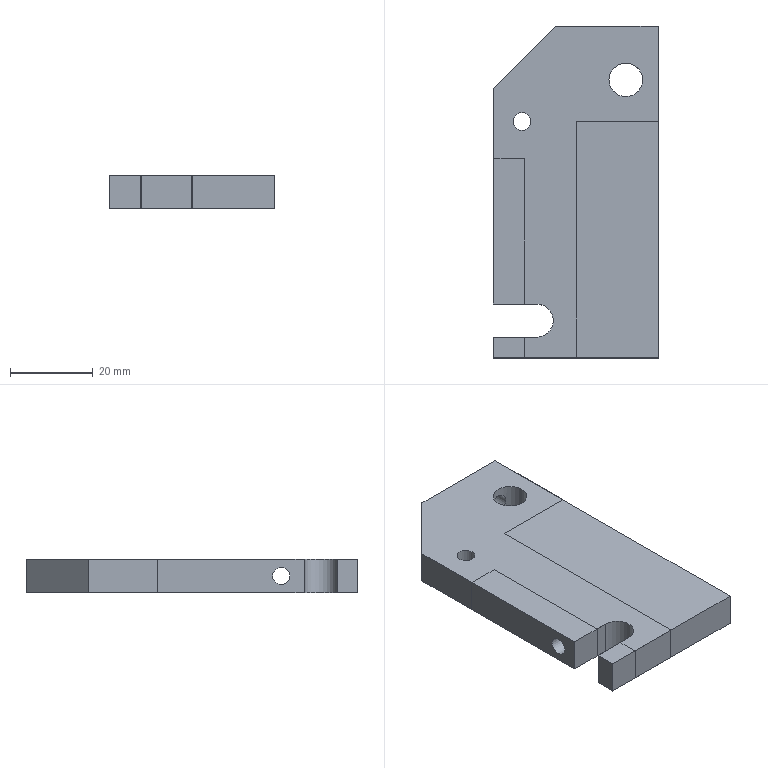NC program | NX | posted with a generic post | part box 40 x 80 x 8 mm
Lines 595 to 1352 of 5028:
(动态粗_COPY , TOOL : D5-15-D6-50-3T-ROUGH)
N1170 T04 M6
N1172 G53
N1174 G17 G0 G90 X34.536 Y-24.337 B0. C0. S3000 M3
N1176 G43 Z20. H4
N1178 Z-9.5
N1180 G94 G1 X34.533 Y-24.312 Z-9.656 F1000.
N1182 X34.531 Y-24.287 Z-9.718
N1184 X34.529 Y-24.262 Z-9.763
N1186 X34.526 Y-24.237 Z-9.8
N1188 X34.524 Y-24.212 Z-9.831
N1190 X34.521 Y-24.187 Z-9.857
N1192 X34.519 Y-24.162 Z-9.88
N1194 X34.517 Y-24.137 Z-9.9
N1196 X34.514 Y-24.113 Z-9.918
N1198 X34.512 Y-24.088 Z-9.933
N1200 X34.51 Y-24.063 Z-9.947
N1202 X34.507 Y-24.038 Z-9.958
N1204 X34.505 Y-24.013 Z-9.968
N1206 X34.503 Y-23.988 Z-9.977
N1208 X34.5 Y-23.963 Z-9.984
N1210 X34.498 Y-23.938 Z-9.99
N1212 X34.496 Y-23.913 Z-9.994
N1214 X34.493 Y-23.889 Z-9.997
N1216 X34.491 Y-23.864 Z-9.999
N1218 X34.488 Y-23.839 Z-10.
N1220 X34.398 Y-22.885
N1222 G3 X34.089 Y-22.466 R0.507
N1224 G2 X33.127 Y-21.874 R2.747
N1226 G3 X28.91 Y-21.835 R3.451
N1228 X28.852 Y-22.496 R0.526
N1230 X29.384 Y-22.726 Z-9.939 R0.57
N1232 G1 X29.771 Y-22.725 Z-9.9
N1234 X32.205 Y-22.72 F10000.
N1236 X32.793 Y-22.712 Z-9.959 F1000.
N1238 G3 X33.133 Y-22.506 Z-10. R0.541
N1240 X33.127 Y-21.874 R0.526
N1242 X30.964 Y-21.083 R2.95
N1244 X28.992 Y-21.722 R3.18
N1246 X28.952 Y-22.359 R0.532
N1248 X29.476 Y-22.602 Z-9.939 R0.578
N1250 G1 X29.866 Y-22.615 Z-9.9
N1252 X32.184 Y-22.694 F10000.
N1254 X32.758 Y-22.707 Z-9.958 F1000.
N1256 G3 X33.114 Y-22.502 Z-10. R0.547
N1258 X33.114 Y-21.856 R0.532
N1260 X31.527 Y-21.067 R2.439
N1262 X29.096 Y-21.59 R3.281
N1264 G2 X27.917 Y-22.464 R2.412
N1266 G3 X29.138 Y-21.545 R2.488
N1268 G2 X32.923 Y-21.618 R3.277
N1270 G1 X32.964 Y-21.662
N1272 G2 X32.995 Y-22.307 R0.551
N1274 X32.426 Y-22.553 Z-9.934 R0.591
N1276 G1 X32.084 Y-22.546 Z-9.9
N1278 X29.975 Y-22.501 F10000.
N1280 X29.418 Y-22.482 Z-9.956 F1000.
N1282 G2 X29.06 Y-22.248 Z-10. R0.566
N1284 X29.08 Y-21.606 R0.551
N1286 X30.487 Y-20.993 R2.3
N1288 X32.897 Y-21.574 R3.091
N1290 G1 X33.061 Y-21.788
N1292 G3 X31.75 Y-20.986 R1.947
N1294 X29.244 Y-21.404 R3.153
N1296 G1 X29.102 Y-21.578
N1298 G2 X30.119 Y-20.975 R1.612
N1300 X32.758 Y-21.406 R3.138
N1302 G1 X32.878 Y-21.549
N1304 G3 X31.663 Y-20.88 R1.861
N1306 X29.343 Y-21.274 R2.987
N1308 G1 X29.297 Y-21.324
N1310 G3 X29.34 Y-21.829 R0.552
N1312 X29.855 Y-22.091 Z-9.939 R0.599
N1314 G1 X30.247 Y-22.124 Z-9.9
N1316 X31.85 Y-22.262 F10000.
N1318 X32.372 Y-22.302 Z-9.953 F1000.
N1320 G3 X32.777 Y-22.088 Z-10. R0.56
N1322 X32.778 Y-21.418 R0.551
N1324 X31.432 Y-20.788 R2.039
N1326 X29.397 Y-21.191 R2.835
N1328 G1 X29.321 Y-21.283
N1330 G3 X29.324 Y-21.864 R0.551
N1332 X29.856 Y-22.125 Z-9.938 R0.593
N1334 G1 X30.23 Y-22.143 Z-9.9
N1336 X31.816 Y-22.221 F10000.
N1338 X32.359 Y-22.24 Z-9.955 F1000.
N1340 G3 X32.739 Y-22.019 Z-10. R0.565
N1342 X32.732 Y-21.359 R0.551
N1344 X31.38 Y-20.727 R2.003
N1346 X29.436 Y-21.121 R2.722
N1348 G1 X29.336 Y-21.242
N1350 G3 X29.369 Y-21.826 R0.551
N1352 X29.907 Y-22.058 Z-9.939 R0.596
N1354 G1 X30.29 Y-22.063 Z-9.9
N1356 X31.707 Y-22.079 F10000.
N1358 X32.277 Z-9.957 F1000.
N1360 G3 X32.635 Y-21.868 Z-10. R0.566
N1362 X32.706 Y-21.325 R0.552
N1364 X31.499 Y-20.693 R1.799
N1366 X29.508 Y-21.024 R2.774
N1368 G1 X29.347 Y-21.207
N1370 G3 X29.409 Y-21.778 R0.52
N1372 X29.89 Y-21.966 Z-9.946 R0.568
N1374 G1 X30.35 Y-21.975 Z-9.9
N1376 X31.655 Y-21.999 F10000.
N1378 X32.241 Y-22.004 Z-9.959 F1000.
N1380 G3 X32.585 Y-21.801 Z-10. R0.534
N1382 X32.569 Y-21.159 R0.519
N1384 X31.042 Y-20.593 R2.168
N1386 X29.454 Y-21.033 R2.294
N1388 G1 X29.365 Y-21.161
N1390 G3 X29.429 Y-21.721 R0.536
N1392 X29.905 Y-21.928 Z-9.946 R0.587
N1394 G1 X30.362 Y-21.958 Z-9.9
N1396 X31.685 Y-22.042 F10000.
N1398 X32.266 Y-22.073 Z-9.959 F1000.
N1400 G3 X32.624 Y-21.888 Z-10. R0.551
N1402 X32.706 Y-21.325 R0.536
N1404 X31.554 Y-20.604 R1.615
N1406 X29.547 Y-20.912 R2.604
N1408 G1 X29.384 Y-21.113
N1410 G3 X29.454 Y-21.655 R0.552
N1412 X29.939 Y-21.88 Z-9.944 R0.607
N1414 G1 X30.379 Y-21.92 Z-9.9
N1416 X31.681 Y-22.04 F10000.
N1418 X32.236 Y-22.084 Z-9.956 F1000.
N1420 G3 X32.617 Y-21.891 Z-10. R0.566
N1422 X32.706 Y-21.325 R0.551
N1424 X31.737 Y-20.603 R1.411
N1426 X29.587 Y-20.841 R2.601
N1428 X29.296 Y-21.325 R0.937
N1430 G1 X29.209 Y-21.438
N1432 G3 X29.457 Y-20.962 R2.18
N1434 G2 X30.727 Y-20.46 R1.779
N1436 X32.538 Y-21.032 R2.348
N1438 G1 X32.645 Y-21.179
N1440 G2 X32.559 Y-21.767 R0.529
N1442 X32.038 Y-21.93 Z-9.943 R0.577
N1444 G1 X31.612 Y-21.9 Z-9.9
N1446 X30.447 Y-21.818 F10000.
N1448 X29.781 Y-21.765 Z-9.967 F1000.
N1450 G2 X29.503 Y-21.6 Z-10. R0.555
N1452 X29.411 Y-21.048 R0.529
N1454 X30.224 Y-20.511 R1.155
N1456 X32.485 Y-20.952 R2.514
N1458 G1 X32.63 Y-21.141
N1460 G2 X32.541 Y-21.717 R0.551
N1462 X31.996 Y-21.902 Z-9.94 R0.599
N1464 G1 X31.602 Y-21.88 Z-9.9
N1466 X30.447 Y-21.817 F10000.
N1468 X30.128 Y-21.801 Z-9.932 F1000.
N1470 X29.809 Y-21.775 Z-9.964
N1472 G2 X29.509 Y-21.594 Z-10. R0.575
N1474 X29.419 Y-21.027 R0.551
N1476 X30.296 Y-20.467 R1.225
N1478 X32.507 Y-20.947 R2.444
N1480 G1 X32.61 Y-21.094
N1482 G2 X32.524 Y-21.675 R0.551
N1484 X31.993 Y-21.862 Z-9.941 R0.595
N1486 G1 X31.584 Y-21.844 Z-9.9
N1488 X30.457 Y-21.797 F10000.
N1490 X30.139 Y-21.785 Z-9.932 F1000.
N1492 X29.821 Y-21.762 Z-9.964
N1494 G2 X29.517 Y-21.583 Z-10. R0.574
N1496 X29.425 Y-21.014 R0.551
N1498 X30.324 Y-20.435 R1.246
N1500 X32.508 Y-20.924 R2.396
N1502 G1 X32.594 Y-21.055
N1504 G2 X32.502 Y-21.624 R0.551
N1506 X31.978 Y-21.812 Z-9.942 R0.597
N1508 G1 X31.562 Y-21.8 Z-9.9
N1510 X30.468 Y-21.769 F10000.
N1512 X30.152 Y-21.761 Z-9.932 F1000.
N1514 X29.836 Y-21.743 Z-9.964
N1516 G2 X29.527 Y-21.564 Z-10. R0.574
N1518 X29.434 Y-20.993 R0.551
N1520 X30.33 Y-20.408 R1.259
N1522 X32.497 Y-20.89 R2.362
N1524 G1 X32.578 Y-21.015
N1526 G2 X32.487 Y-21.583 R0.551
N1528 X31.966 Y-21.773 Z-9.942 R0.598
N1530 G1 X31.547 Y-21.765 Z-9.9
N1532 X30.478 Y-21.743 F10000.
N1534 X30.163 Y-21.738 Z-9.932 F1000.
N1536 X29.849 Y-21.723 Z-9.963
N1538 G2 X29.537 Y-21.545 Z-10. R0.574
N1540 X29.442 Y-20.972 R0.551
N1542 X30.375 Y-20.372 R1.291
N1544 X32.483 Y-20.852 R2.321
N1546 X32.678 Y-21.256 R4.312
N1548 G3 X31.725 Y-20.375 R1.255
N1550 X29.64 Y-20.67 R2.289
N1552 X29.448 Y-20.957 R0.882
N1554 G2 X30.232 Y-20.336 R1.083
N1556 X32.434 Y-20.757 R2.275
N1558 G1 X32.549 Y-20.946
N1560 G3 X31.73 Y-20.304 R1.206
N1562 X29.629 Y-20.625 R2.189
N1564 G1 X29.491 Y-20.854
N1566 G2 X30.235 Y-20.264 R1.049
N1568 X32.4 Y-20.675 R2.198
N1570 G1 X32.519 Y-20.873
N1572 G3 X31.679 Y-20.216 R1.209
N1574 X29.659 Y-20.545 R2.117
N1576 G1 X29.528 Y-20.766
N1578 G2 X30.274 Y-20.18 R1.04
N1580 X32.381 Y-20.61 R2.114
N1582 G1 X32.482 Y-20.784
N1584 G3 X31.602 Y-20.123 R1.23
N1586 X29.671 Y-20.484 R2.016
N1588 G1 X29.569 Y-20.658
N1590 G3 X29.677 Y-21.153 R0.552
N1592 X30.166 Y-21.357 Z-9.945 R0.609
N1594 G1 X30.612 Y-21.383 Z-9.9
N1596 X31.394 Y-21.43 F10000.
N1598 X31.987 Y-21.459 Z-9.96 F1000.
N1600 G3 X32.341 Y-21.288 Z-10. R0.568
N1602 X32.448 Y-20.701 R0.551
N1604 X31.472 Y-20.046 R1.339
N1606 X29.678 Y-20.439 R1.943
N1608 G1 X29.576 Y-20.622
N1610 G3 X29.695 Y-21.148 R0.549
N1612 X30.204 Y-21.326 Z-9.944 R0.6
N1614 G1 X30.64 Y-21.32 Z-9.9
N1616 X31.346 Y-21.311 F10000.
N1618 X31.67 Y-21.307 Z-9.933 F1000.
N1620 X31.993 Y-21.295 Z-9.965
N1622 G3 X32.296 Y-21.133 Z-10. R0.572
N1624 X32.442 Y-20.686 R0.55
N1626 X31.556 Y-20.024 R1.241
N1628 X29.696 Y-20.383 R1.939
N1630 G1 X29.577 Y-20.597
N1632 G3 X29.709 Y-21.091 R0.514
N1634 X30.153 Y-21.244 Z-9.952 R0.574
N1636 G1 X30.665 Y-21.256 Z-9.9
N1638 X31.329 Y-21.273 F10000.
N1640 X31.998 Y-21.283 Z-9.967 F1000.
N1642 G3 X32.287 Y-21.142 Z-10. R0.538
N1644 X32.418 Y-20.62 R0.514
N1646 X31.397 Y-19.943 R1.356
N1648 X29.686 Y-20.357 R1.845
N1650 G1 X29.579 Y-20.569
N1652 G3 X29.725 Y-21.058 R0.518
N1654 X30.167 Y-21.202 Z-9.952 R0.579
N1656 G1 X30.684 Y-21.211 Z-9.9
N1658 X31.307 Y-21.221 F10000.
N1660 X31.633 Y-21.228 Z-9.933 F1000.
N1662 X31.959 Y-21.224 Z-9.965
N1664 G3 X32.258 Y-21.067 Z-10. R0.539
N1666 X32.329 Y-20.459 R0.516
N1668 X30.976 Y-19.851 R1.633
N1670 X29.643 Y-20.379 R1.575
N1672 G1 X29.583 Y-20.532
N1674 G3 X29.733 Y-21.015 R0.521
N1676 X30.156 Y-21.163 Z-9.954 R0.592
N1678 G1 X30.691 Y-21.196 Z-9.9
N1680 X31.314 Y-21.235 F10000.
N1682 X31.642 Y-21.256 Z-9.933 F1000.
N1684 X31.971 Y-21.268 Z-9.966
N1686 G3 X32.273 Y-21.13 Z-10. R0.543
N1688 X32.422 Y-20.628 R0.521
N1690 X31.467 Y-19.874 R1.249
N1692 X29.705 Y-20.258 R1.83
N1694 X29.586 Y-20.497 R1.8
N1696 X29.742 Y-20.978 R0.533
N1698 X30.16 Y-21.132 Z-9.954 R0.611
N1700 G1 X30.698 Y-21.18 Z-9.9
N1702 X31.315 Y-21.235 F10000.
N1704 X31.635 Y-21.265 Z-9.932 F1000.
N1706 X31.956 Y-21.285 Z-9.965
N1708 G3 X32.274 Y-21.147 Z-10. R0.555
N1710 X32.442 Y-20.686 R0.534
N1712 X31.634 Y-19.885 R1.114
N1714 X29.717 Y-20.206 R1.85
N1716 X29.591 Y-20.458 R1.211
N1718 X29.754 Y-20.945 R0.552
N1720 X30.179 Y-21.104 Z-9.953 R0.626
N1722 G1 X30.708 Y-21.154 Z-9.9
N1724 X31.304 Y-21.21 F10000.
N1726 X31.915 Y-21.262 Z-9.962 F1000.
N1728 G3 X32.262 Y-21.118 Z-10. R0.57
N1730 X32.436 Y-20.641 R0.552
N1732 X31.664 Y-19.856 R1.1
N1734 X29.728 Y-20.155 R1.842
N1736 X29.596 Y-20.419 R0.959
N1738 X29.769 Y-20.896 R0.552
N1740 X30.184 Y-21.048 Z-9.955 R0.635
N1742 G1 X30.726 Y-21.103 Z-9.9
N1744 X31.284 Y-21.16 F10000.
N1746 X31.601 Y-21.194 Z-9.932 F1000.
N1748 X31.918 Y-21.217 Z-9.964
N1750 G3 X32.245 Y-21.084 Z-10. R0.574
N1752 X32.43 Y-20.597 R0.552
N1754 X31.662 Y-19.815 R1.107
N1756 X29.731 Y-20.113 R1.821
N1758 X29.561 Y-20.686 R0.896
N1760 G2 X29.783 Y-20.045 R0.909
N1762 X32.305 Y-20.259 R1.829
N1764 G1 X32.416 Y-20.496
N1766 G2 X32.233 Y-21.001 R0.533
N1768 X31.751 Y-21.113 Z-9.949 R0.593
N1770 G1 X31.268 Y-21.071 Z-9.9
N1772 X30.767 Y-21.027 F10000.
N1774 X30.006 Y-20.955 Z-9.977 F1000.
N1776 X29.898 Y-20.913 Z-9.988
N1778 X29.799 Y-20.854 Z-10.
N1780 G2 X29.603 Y-20.369 R0.533
N1782 X30.219 Y-19.756 R0.872
N1784 X32.325 Y-20.262 R1.822
N1786 G1 X32.412 Y-20.467
N1788 G2 X32.228 Y-20.973 R0.552
N1790 X31.734 Y-21.097 Z-9.947 R0.609
N1792 G1 X31.265 Y-21.062 Z-9.9
N1794 X30.767 Y-21.024 F10000.
N1796 X30.026 Y-20.961 Z-9.975 F1000.
N1798 X29.908 Y-20.917 Z-9.987
N1800 X29.802 Y-20.851 Z-10.
N1802 G2 X29.605 Y-20.354 R0.552
N1804 X30.283 Y-19.711 R0.922
N1806 X32.338 Y-20.253 R1.803
N1808 G1 X32.408 Y-20.434
N1810 G2 X32.219 Y-20.942 R0.552
N1812 X31.734 Y-21.064 Z-9.948 R0.612
N1814 G1 X31.255 Y-21.033 Z-9.9
N1816 X30.774 Y-21.002 F10000.
N1818 X30.033 Y-20.948 Z-9.975 F1000.
N1820 X29.914 Y-20.904 Z-9.987
N1822 X29.807 Y-20.839 Z-10.
N1824 G2 X29.607 Y-20.339 R0.552
N1826 X30.315 Y-19.679 R0.95
N1828 X32.335 Y-20.224 R1.792
N1830 G1 X32.405 Y-20.406
N1832 G2 X32.211 Y-20.909 R0.552
N1834 X31.734 Y-21.03 Z-9.949 R0.616
N1836 G1 X31.245 Y-21.004 Z-9.9
N1838 X30.778 Y-20.979 F10000.
N1840 X30.409 Y-20.961 Z-9.937 F1000.
N1842 X30.04 Y-20.934 Z-9.974
N1844 X29.92 Y-20.891 Z-9.987
N1846 X29.81 Y-20.825 Z-10.
N1848 G2 X29.609 Y-20.324 R0.552
N1850 X30.321 Y-19.655 R0.958
N1852 X32.332 Y-20.194 R1.785
N1854 G1 X32.401 Y-20.375
N1856 G2 X32.205 Y-20.871 R0.552
N1858 X31.735 Y-20.992 Z-9.95 R0.619
N1860 G1 X31.239 Y-20.973 Z-9.9
N1862 X30.782 Y-20.955 F10000.
N1864 X30.415 Y-20.943 Z-9.937 F1000.
N1866 X30.048 Y-20.92 Z-9.974
N1868 X29.925 Y-20.878 Z-9.987
N1870 X29.813 Y-20.811 Z-10.
N1872 G2 X29.611 Y-20.309 R0.552
N1874 X30.308 Y-19.639 R0.958
N1876 X32.332 Y-20.171 R1.774
N1878 G1 X32.397 Y-20.346
N1880 G2 X32.201 Y-20.842 R0.552
N1882 X31.742 Y-20.964 Z-9.951 R0.615
N1884 G1 X31.234 Y-20.949 Z-9.9
N1886 X30.786 Y-20.935 F10000.
N1888 X30.42 Y-20.926 Z-9.937 F1000.
N1890 X30.054 Y-20.906 Z-9.974
N1892 X29.93 Y-20.864 Z-9.987
N1894 X29.817 Y-20.797 Z-10.
N1896 G2 X29.613 Y-20.294 R0.552
N1898 X30.307 Y-19.618 R0.962
N1900 X32.327 Y-20.138 R1.768
N1902 X32.424 Y-20.553 R1.39
N1904 G3 X31.759 Y-19.64 R0.978
N1906 X29.759 Y-19.938 R1.756
N1908 X29.615 Y-20.275 R0.687
N1910 G2 X30.227 Y-19.587 R0.876
N1912 X32.313 Y-20.066 R1.753
N1914 G1 X32.385 Y-20.254
N1916 G2 X32.184 Y-20.754 R0.552
N1918 X31.729 Y-20.872 Z-9.952 R0.617
N1920 G1 X31.215 Y-20.856 Z-9.9
N1922 X30.804 Y-20.843 F10000.
N1924 X30.435 Y-20.832 Z-9.937 F1000.
N1926 X30.067 Y-20.813 Z-9.974
N1928 X29.945 Y-20.772 Z-9.987
N1930 X29.834 Y-20.707 Z-10.
N1932 G2 X29.625 Y-20.2 R0.552
N1934 X30.32 Y-19.529 R0.97
N1936 X32.311 Y-20.038 R1.742
N1938 X32.39 Y-20.296 R2.963
N1940 G3 X31.78 Y-19.562 R0.93
N1942 X29.743 Y-19.884 R1.721
N1944 X29.627 Y-20.187 R0.802
N1946 G2 X30.239 Y-19.498 R0.878
N1948 X32.297 Y-19.966 R1.732
N1950 G1 X32.378 Y-20.205
N1952 G3 X31.75 Y-19.484 R0.952
N1954 X29.767 Y-19.796 R1.724
N1956 X29.636 Y-20.119 R0.727
N1958 G2 X30.237 Y-19.437 R0.868
N1960 X32.29 Y-19.903 R1.712
N1962 G1 X32.37 Y-20.145
N1964 G3 X31.72 Y-19.408 R0.964
N1966 X29.743 Y-19.77 R1.684
N1968 G1 X29.651 Y-19.997
N1970 G3 X29.857 Y-20.426 R0.553
N1972 X30.247 Y-20.553 Z-9.958 R0.643
N1974 G1 X30.823 Y-20.605 Z-9.9
N1976 X31.174 Y-20.637 F10000.
N1978 X31.846 Y-20.692 Z-9.968 F1000.
N1980 G3 X32.145 Y-20.583 Z-10. R0.58
N1982 X32.361 Y-20.071 R0.552
N1984 X31.611 Y-19.324 R1.054
N1986 X29.742 Y-19.729 R1.663
N1988 X29.652 Y-19.98 R1.837
N1990 X29.856 Y-20.439 R0.553
N1992 X30.262 Y-20.565 Z-9.956 R0.633
N1994 G1 X30.823 Y-20.598 Z-9.9
N1996 X31.171 Y-20.618 F10000.
N1998 X31.856 Y-20.653 Z-9.969 F1000.
N2000 G3 X32.142 Y-20.544 Z-10. R0.583
N2002 X32.356 Y-20.034 R0.552
N2004 X31.611 Y-19.286 R1.058
N2006 X29.745 Y-19.685 R1.655
N2008 X29.652 Y-19.951 R1.206
N2010 X29.861 Y-20.4 R0.54
N2012 X30.274 Y-20.512 Z-9.956 R0.617
N2014 G1 X30.833 Y-20.521 Z-9.9
N2016 X31.159 Y-20.526 F10000.
N2018 X31.526 Y-20.533 Z-9.937 F1000.
N2020 X31.893 Y-20.53 Z-9.974
N2022 X32.018 Y-20.493 Z-9.987
N2024 X32.132 Y-20.431 Z-10.
N2026 G3 X32.351 Y-19.999 R0.54
N2028 X31.584 Y-19.238 R1.068
N2030 X29.742 Y-19.649 R1.638
N2032 X29.651 Y-19.915 R1.21
N2034 X29.865 Y-20.366 R0.553
N2036 X30.272 Y-20.484 Z-9.957 R0.634
N2038 G1 X30.835 Y-20.508 Z-9.9
N2040 X31.158 Y-20.522 F10000.
N2042 X31.853 Y-20.546 Z-9.97 F1000.
N2044 G3 X32.13 Y-20.439 Z-10. R0.586
N2046 X32.351 Y-19.999 R0.553
N2048 X31.679 Y-19.238 R0.991
N2050 X29.755 Y-19.59 R1.658
N2052 X29.651 Y-19.882 R0.821
N2054 X29.869 Y-20.321 R0.553
N2056 X30.258 Y-20.438 Z-9.959 R0.646
N2058 G1 X30.84 Y-20.48 Z-9.9
N2060 X31.156 Y-20.503 F10000.
N2062 X31.839 Y-20.548 Z-9.969 F1000.
N2064 G3 X32.128 Y-20.441 Z-10. R0.583
N2066 X32.351 Y-19.999 R0.553
N2068 X31.746 Y-19.231 R0.937
N2070 X29.773 Y-19.525 R1.676
N2072 X29.651 Y-19.84 R0.714
N2074 X29.874 Y-20.282 R0.553
N2076 X30.257 Y-20.396 Z-9.959 R0.651
N2078 G1 X30.845 Y-20.44 Z-9.9
N2080 X31.151 Y-20.464 F10000.
N2082 X31.837 Y-20.51 Z-9.969 F1000.
N2084 G3 X32.124 Y-20.407 Z-10. R0.584
N2086 X32.351 Y-19.962 R0.553
N2088 X31.722 Y-19.181 R0.963
N2090 X29.759 Y-19.502 R1.655
N2092 X29.645 Y-20.046 R0.821
N2094 G2 X30.241 Y-19.125 R0.844
N2096 X32.268 Y-19.631 R1.654
N2098 X32.351 Y-19.892 R1.877
N2100 X32.127 Y-20.343 R0.553
N2102 X31.671 Y-20.443 Z-9.952 R0.618
N2104 G1 X31.155 Y-20.408 Z-9.9
N2106 X30.863 Y-20.389 F10000.
N2108 X30.091 Y-20.332 Z-9.978 F1000.
N2110 X29.986 Y-20.296 Z-9.989
N2112 X29.888 Y-20.245 Z-10.
N2114 G2 X29.651 Y-19.793 R0.552
N2116 X30.219 Y-19.115 R0.828
N2118 X32.258 Y-19.588 R1.665
N2120 X32.351 Y-19.869 R1.078
N2122 X32.125 Y-20.314 R0.553
N2124 X31.675 Y-20.413 Z-9.953 R0.622
N2126 G1 X31.152 Y-20.383 Z-9.9
N2128 X30.865 Y-20.367 F10000.
N2130 X30.096 Y-20.318 Z-9.978 F1000.
N2132 X29.989 Y-20.283 Z-9.989
N2134 X29.89 Y-20.231 Z-10.
N2136 G2 X29.651 Y-19.778 R0.552
N2138 X30.247 Y-19.082 R0.856
N2140 X32.278 Y-19.593 R1.647
N2142 X32.351 Y-19.842 R2.599
N2144 X32.122 Y-20.288 R0.553
N2146 X31.678 Y-20.386 Z-9.953 R0.625
N2148 G1 X31.148 Y-20.36 Z-9.9
N2150 X30.868 Y-20.346 F10000.
N2152 X30.099 Y-20.303 Z-9.977 F1000.
N2154 X29.992 Y-20.269 Z-9.989
N2156 X29.892 Y-20.218 Z-10.
N2158 G2 X29.651 Y-19.763 R0.552
N2160 X30.268 Y-19.053 R0.877
N2162 X32.283 Y-19.574 R1.644
N2164 G1 X32.351 Y-19.809
N2166 G2 X32.12 Y-20.257 R0.553
N2168 X31.683 Y-20.354 Z-9.954 R0.631
N2170 G1 X31.145 Y-20.334 Z-9.9
N2172 X30.871 Y-20.324 F10000.
N2174 X30.104 Y-20.289 Z-9.977 F1000.
N2176 X29.996 Y-20.255 Z-9.989
N2178 X29.894 Y-20.204 Z-10.
N2180 G2 X29.651 Y-19.748 R0.552
N2182 X30.255 Y-19.038 R0.881
N2184 X32.287 Y-19.554 R1.642
N2186 G1 X32.351 Y-19.783
N2188 G2 X32.117 Y-20.233 R0.552
N2190 X31.685 Y-20.329 Z-9.955 R0.634
N2192 G1 X31.142 Y-20.312 Z-9.9
N2194 X30.873 Y-20.304 F10000.
N2196 X30.108 Y-20.275 Z-9.977 F1000.
N2198 X29.998 Y-20.242 Z-9.988
N2200 X29.896 Y-20.19 Z-10.
N2202 G2 X29.651 Y-19.733 R0.552
N2204 X30.255 Y-19.018 R0.887
N2206 X32.293 Y-19.538 R1.635
N2208 X32.351 Y-19.937 R0.952
N2210 G3 X31.832 Y-19.058 R0.87
N2212 X29.76 Y-19.364 R1.632
N2214 X29.651 Y-19.661 R0.838
N2216 X29.894 Y-20.117 R0.552
N2218 X30.275 Y-20.215 Z-9.96 R0.656
N2220 G1 X30.871 Y-20.242 Z-9.9
N2222 X31.123 Y-20.254 F10000.
N2224 X31.492 Y-20.273 Z-9.937 F1000.
N2226 X31.862 Y-20.282 Z-9.974
N2228 X31.986 Y-20.251 Z-9.987
N2230 X32.102 Y-20.195 Z-10.
N2232 G3 X32.351 Y-19.735 R0.552
N2234 X31.767 Y-18.985 R0.929
N2236 X29.756 Y-19.325 R1.63
N2238 X29.651 Y-19.615 R0.88
N2240 X29.898 Y-20.08 R0.552
N2242 X30.313 Y-20.178 Z-9.957 R0.751
N2244 G1 X30.875 Y-20.207 Z-9.9
N2246 X31.119 Y-20.22 F10000.
N2248 X31.488 Y-20.241 Z-9.937 F1000.
N2250 X31.858 Y-20.252 Z-9.974
N2252 X31.982 Y-20.222 Z-9.987
N2254 X32.098 Y-20.168 Z-10.
N2256 G3 X32.351 Y-19.705 R0.552
N2258 X31.723 Y-18.925 R0.961
N2260 X29.741 Y-19.301 R1.618
N2262 X29.653 Y-19.545 R2.581
N2264 X29.9 Y-20.031 R0.52
N2266 X30.291 Y-20.114 Z-9.959 R0.769
N2268 G1 X30.882 Y-20.145 Z-9.9
N2270 X31.11 Y-20.157 F10000.
N2272 X31.881 Y-20.191 Z-9.977 F1000.
N2274 X31.99 Y-20.167 Z-9.989
N2276 X32.093 Y-20.123 Z-10.
N2278 G3 X32.351 Y-19.675 R0.521
N2280 X31.732 Y-18.892 R0.963
N2282 X29.74 Y-19.258 R1.62
N2284 X29.653 Y-19.503 R2.577
N2286 X29.903 Y-19.989 R0.52
N2288 X30.278 Y-20.07 Z-9.961 R0.763
N2290 G1 X30.884 Y-20.107 Z-9.9
N2292 X31.108 Y-20.121 F10000.
N2294 X31.877 Y-20.162 Z-9.977 F1000.
N2296 X31.987 Y-20.138 Z-9.989
N2298 X32.091 Y-20.094 Z-10.
N2300 G3 X32.351 Y-19.645 R0.521
N2302 X31.701 Y-18.839 R0.981
N2304 X29.739 Y-19.217 R1.617
N2306 X29.653 Y-19.462 R2.587
N2308 X29.905 Y-19.949 R0.523
N2310 X30.28 Y-20.03 Z-9.961 R0.771
N2312 G1 X30.887 Y-20.07 Z-9.9
N2314 X31.106 Y-20.084 F10000.
N2316 X31.872 Y-20.128 Z-9.977 F1000.
N2318 X31.983 Y-20.103 Z-9.989
N2320 X32.089 Y-20.06 Z-10.
N2322 G3 X32.351 Y-19.607 R0.524
N2324 X31.708 Y-18.804 R0.986
N2326 X29.74 Y-19.172 R1.619
N2328 X29.653 Y-19.417 R2.58
N2330 X29.908 Y-19.905 R0.52
N2332 X30.276 Y-19.985 Z-9.962 R0.781
N2334 G1 X30.89 Y-20.026 Z-9.9
N2336 X31.103 Y-20.04 F10000.
N2338 X31.873 Y-20.087 Z-9.977 F1000.
N2340 X31.982 Y-20.064 Z-9.989
N2342 X32.086 Y-20.022 Z-10.
N2344 G3 X32.351 Y-19.57 R0.521
N2346 X31.675 Y-18.751 R1.008
N2348 X29.737 Y-19.135 R1.612
N2350 G1 X29.653 Y-19.373
N2352 G3 X29.909 Y-19.864 R0.52
N2354 X30.274 Y-19.943 Z-9.962 R0.794
N2356 G1 X30.891 Y-19.989 Z-9.9
N2358 X31.101 Y-20.005 F10000.
N2360 X31.869 Y-20.057 Z-9.977 F1000.
N2362 X31.979 Y-20.035 Z-9.989
N2364 X32.084 Y-19.993 Z-10.
N2366 G3 X32.351 Y-19.54 R0.52
N2368 X31.707 Y-18.727 R0.994
N2370 X29.743 Y-19.083 R1.62
N2372 X29.653 Y-19.335 R1.781
N2374 X29.91 Y-19.823 R0.523
N2376 X30.275 Y-19.904 Z-9.962 R0.797
N2378 G1 X30.892 Y-19.952 Z-9.9
N2380 X31.1 Y-19.969 F10000.
N2382 X31.865 Y-20.023 Z-9.977 F1000.
N2384 X31.977 Y-20. Z-9.989
N2386 X32.083 Y-19.958 Z-10.
N2388 G3 X32.351 Y-19.502 R0.524
N2390 X31.682 Y-18.677 R1.011
N2392 X29.74 Y-19.045 R1.614
N2394 X29.653 Y-19.29 R2.577
N2396 X29.91 Y-19.779 R0.52
N2398 X30.271 Y-19.859 Z-9.963 R0.801
N2400 G1 X30.892 Y-19.909 Z-9.9
N2402 X31.1 Y-19.926 F10000.
N2404 X31.867 Y-19.983 Z-9.977 F1000.
N2406 X31.978 Y-19.96 Z-9.989
N2408 X32.084 Y-19.919 Z-10.
N2410 G3 X32.351 Y-19.465 R0.52
N2412 X31.692 Y-18.644 R1.011
N2414 X29.744 Y-18.997 R1.619
N2416 X29.653 Y-19.248 R1.777
N2418 X29.91 Y-19.737 R0.52
N2420 X30.27 Y-19.817 Z-9.963 R0.804
N2422 G1 X30.892 Y-19.869 Z-9.9
N2424 X31.101 Y-19.887 F10000.
N2426 X31.866 Y-19.945 Z-9.977 F1000.
N2428 X31.977 Y-19.923 Z-9.989
N2430 X32.084 Y-19.881 Z-10.
N2432 G3 X32.351 Y-19.427 R0.52
N2434 X31.666 Y-18.594 R1.027
N2436 X29.738 Y-18.965 R1.607
N2438 G1 X29.653 Y-19.203
N2440 G3 X29.91 Y-19.697 R0.52
N2442 X30.267 Y-19.777 Z-9.963 R0.812
N2444 G1 X30.892 Y-19.834 Z-9.9
N2446 X31.1 Y-19.852 F10000.
N2448 X31.863 Y-19.915 Z-9.977 F1000.
N2450 X31.976 Y-19.893 Z-9.988
N2452 X32.083 Y-19.852 Z-10.
N2454 G3 X32.351 Y-19.397 R0.52
N2456 X31.671 Y-18.557 R1.023
N2458 X29.745 Y-18.913 R1.614
N2460 X29.653 Y-19.164 R1.774
N2462 X29.911 Y-19.655 R0.52
N2464 X30.266 Y-19.736 Z-9.963 R0.816
N2466 G1 X30.892 Y-19.794 Z-9.9
N2468 X31.101 Y-19.813 F10000.
N2470 X31.862 Y-19.878 Z-9.977 F1000.
N2472 X31.975 Y-19.856 Z-9.988
N2474 X32.083 Y-19.814 Z-10.
N2476 G3 X32.351 Y-19.36 R0.52
N2478 X31.693 Y-18.529 R1.016
N2480 X29.75 Y-18.866 R1.618
N2482 X29.653 Y-19.122 R1.404
N2484 X29.911 Y-19.615 R0.52
N2486 X30.266 Y-19.695 Z-9.963 R0.819
N2488 G1 X30.892 Y-19.754 Z-9.9
N2490 X31.101 Y-19.774 F10000.
N2492 X31.861 Y-19.84 Z-9.977 F1000.
N2494 X31.975 Y-19.819 Z-9.988
N2496 X32.083 Y-19.777 Z-10.
N2498 G3 X32.351 Y-19.322 R0.52
N2500 X31.664 Y-18.477 R1.032
N2502 X29.749 Y-18.826 R1.611
N2504 X29.653 Y-19.083 R1.405
N2506 X29.911 Y-19.574 R0.52
N2508 X30.265 Y-19.654 Z-9.963 R0.822
N2510 G1 X30.892 Y-19.715 Z-9.9
N2512 X31.101 Y-19.735 F10000.
N2514 X31.86 Y-19.803 Z-9.977 F1000.
N2516 X31.975 Y-19.781 Z-9.988
N2518 X32.083 Y-19.739 Z-10.
N2520 G3 X32.351 Y-19.285 R0.52
N2522 X31.667 Y-18.44 R1.033
N2524 X29.747 Y-18.788 R1.608
N2526 X29.653 Y-19.038 R1.77
N2528 X29.911 Y-19.533 R0.52
N2530 X30.264 Y-19.614 Z-9.963 R0.825
N2532 G1 X30.892 Y-19.676 Z-9.9
N2534 X31.101 Y-19.696 F10000.
N2536 X31.86 Y-19.765 Z-9.977 F1000.
N2538 X31.974 Y-19.744 Z-9.988
N2540 X32.083 Y-19.702 Z-10.
N2542 G3 X32.351 Y-19.247 R0.52
N2544 X31.675 Y-18.406 R1.032
N2546 X29.747 Y-18.747 R1.608
N2548 X29.653 Y-18.997 R1.769
N2550 X29.911 Y-19.492 R0.52
N2552 X30.263 Y-19.573 Z-9.963 R0.828
N2554 G1 X30.892 Y-19.637 Z-9.9
N2556 X31.101 Y-19.658 F10000.
N2558 X31.859 Y-19.728 Z-9.977 F1000.
N2560 X31.974 Y-19.707 Z-9.988
N2562 X32.083 Y-19.664 Z-10.
N2564 G3 X32.351 Y-19.21 R0.52
N2566 X31.676 Y-18.367 R1.033
N2568 X29.751 Y-18.701 R1.611
N2570 X29.653 Y-18.956 R1.402
N2572 X29.912 Y-19.452 R0.52
N2574 X30.262 Y-19.533 Z-9.964 R0.831
N2576 G1 X30.892 Y-19.597 Z-9.9
N2578 X31.101 Y-19.619 F10000.
N2580 X31.858 Y-19.691 Z-9.976 F1000.
N2582 X31.973 Y-19.669 Z-9.988
N2584 X32.083 Y-19.627 Z-10.
N2586 G3 X32.351 Y-19.172 R0.52
N2588 X31.681 Y-18.331 R1.034
N2590 X29.751 Y-18.66 R1.61
N2592 X29.653 Y-18.915 R1.402
N2594 X29.912 Y-19.411 R0.52
N2596 X30.261 Y-19.492 Z-9.964 R0.834
N2598 G1 X30.892 Y-19.558 Z-9.9
N2600 X31.101 Y-19.58 F10000.
N2602 X31.857 Y-19.653 Z-9.976 F1000.
N2604 X31.973 Y-19.632 Z-9.988
N2606 X32.082 Y-19.589 Z-10.
N2608 G3 X32.351 Y-19.135 R0.52
N2610 X31.678 Y-18.291 R1.037
N2612 X29.751 Y-18.619 R1.608
N2614 X29.653 Y-18.875 R1.402
N2616 X29.912 Y-19.37 R0.52
N2618 X30.261 Y-19.452 Z-9.964 R0.837
N2620 G1 X30.892 Y-19.519 Z-9.9
N2622 X31.101 Y-19.541 F10000.
N2624 X31.856 Y-19.616 Z-9.976 F1000.
N2626 X31.972 Y-19.594 Z-9.988
N2628 X32.082 Y-19.552 Z-10.
N2630 G3 X32.351 Y-19.097 R0.52
N2632 X31.654 Y-18.241 R1.049
N2634 X29.75 Y-18.58 R1.605
N2636 X29.653 Y-18.837 R1.405
N2638 X29.912 Y-19.329 R0.52
N2640 X30.26 Y-19.41 Z-9.964 R0.841
N2642 G1 X30.892 Y-19.479 Z-9.9
N2644 X31.101 Y-19.502 F10000.
N2646 X31.855 Y-19.578 Z-9.976 F1000.
N2648 X31.972 Y-19.557 Z-9.988
N2650 X32.082 Y-19.515 Z-10.
N2652 G3 X32.351 Y-19.06 R0.52
N2654 X31.679 Y-18.214 R1.039
N2656 X29.753 Y-18.535 R1.61
N2658 X29.653 Y-18.797 R1.194
N2660 X29.912 Y-19.288 R0.52
N2662 X30.259 Y-19.37 Z-9.964 R0.844
N2664 G1 X30.892 Y-19.44 Z-9.9
N2666 X31.101 Y-19.463 F10000.
N2668 X31.855 Y-19.541 Z-9.976 F1000.
N2670 X31.971 Y-19.52 Z-9.988
N2672 X32.082 Y-19.477 Z-10.
N2674 G3 X32.351 Y-19.022 R0.52
N2676 X31.655 Y-18.164 R1.051
N2678 X29.747 Y-18.502 R1.601